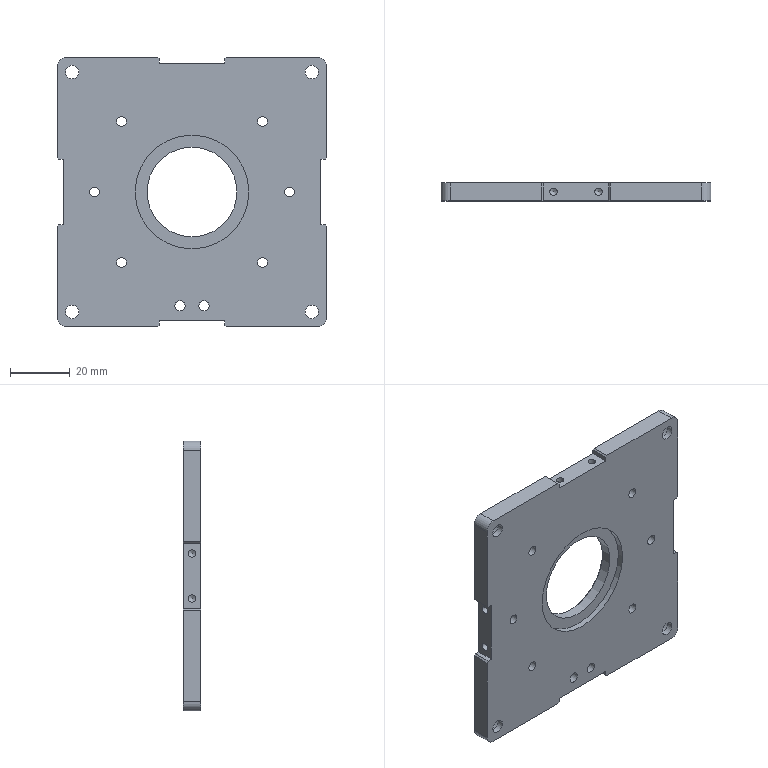Part | NX | 1 solid | 78 faces | box 90 x 6 x 90 mm | volume 40536 mm3 | plane 37 | cylinder 32 | cone 9 | commonest cylinder face diameters 2.5 x8 3.3 x6 4.5 x4 6 x4 8 x4 3.4 x2